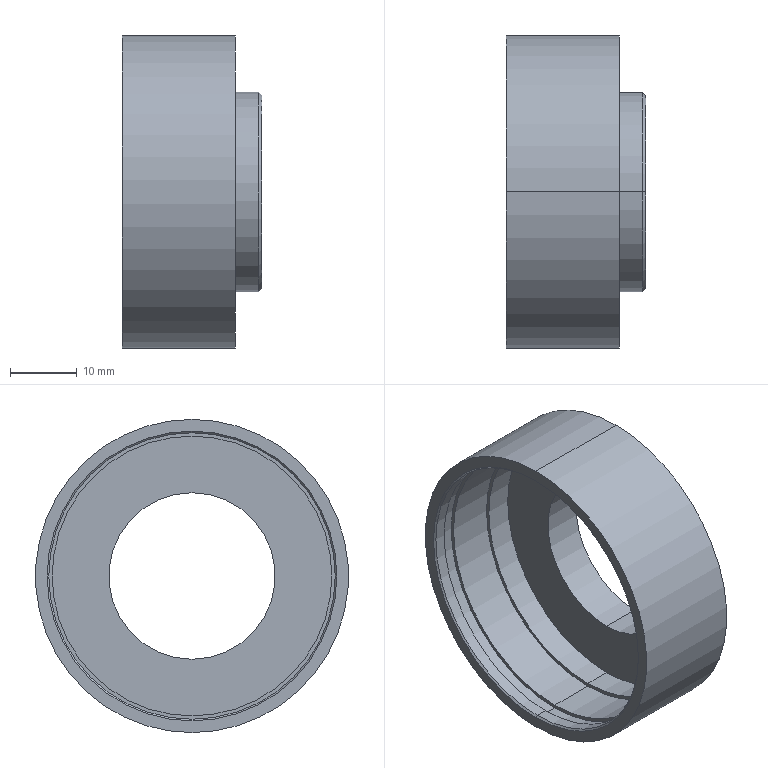Part | SolidWorks | features Chamfer 2, Revolution 1 | 1 solid | 25 faces | box 21 x 47 x 47 mm | volume 7708 mm3 | cylinder 14 | plane 7 | cone 4 | commonest cylinder face diameters 43 x4 25 x2 30 x2 42 x2 44 x2 47 x2
STEP:
#1=CARTESIAN_POINT('',(23.18,0.,-14.5));
#2=VERTEX_POINT('',#1);
#3=CARTESIAN_POINT('',(23.18,0.,14.5));
#4=VERTEX_POINT('',#3);
#5=CARTESIAN_POINT('',(23.18,0.,0.));
#6=DIRECTION('',(1.,0.,0.));
#7=DIRECTION('',(0.,0.,1.));
#8=AXIS2_PLACEMENT_3D('',#5,#6,#7);
#9=CIRCLE('',#8,14.5);
#10=EDGE_CURVE('',#2,#4,#9,.T.);
#11=ORIENTED_EDGE('',*,*,#10,.F.);
#12=CARTESIAN_POINT('',(22.68,0.,-15.));
#13=VERTEX_POINT('',#12);
#14=CARTESIAN_POINT('',(22.68,0.,-15.));
#15=DIRECTION('',(-0.7071,0.,-0.7071));
#16=VECTOR('',#15,1000.);
#17=LINE('',#14,#16);
#18=EDGE_CURVE('',#2,#13,#17,.T.);
#19=ORIENTED_EDGE('',*,*,#18,.T.);
#20=CARTESIAN_POINT('',(22.68,0.,15.));
#21=VERTEX_POINT('',#20);
#22=CARTESIAN_POINT('',(22.68,0.,0.));
#23=DIRECTION('',(-1.,0.,0.));
#24=DIRECTION('',(0.,0.,1.));
#25=AXIS2_PLACEMENT_3D('',#22,#23,#24);
#26=CIRCLE('',#25,15.);
#27=EDGE_CURVE('',#21,#13,#26,.T.);
#28=ORIENTED_EDGE('',*,*,#27,.F.);
#29=CARTESIAN_POINT('',(22.68,0.,15.));
#30=DIRECTION('',(-0.7071,0.,0.7071));
#31=VECTOR('',#30,1000.);
#32=LINE('',#29,#31);
#33=EDGE_CURVE('',#4,#21,#32,.T.);
#34=ORIENTED_EDGE('',*,*,#33,.F.);
#35=EDGE_LOOP('',(#11,#19,#28,#34));
#36=FACE_OUTER_BOUND('',#35,.T.);
#37=CARTESIAN_POINT('',(22.68,0.,0.));
#38=DIRECTION('',(-1.,0.,0.));
#39=DIRECTION('',(0.,0.,1.));
#40=AXIS2_PLACEMENT_3D('',#37,#38,#39);
#41=CONICAL_SURFACE('',#40,15.,0.7854);
#42=ADVANCED_FACE('',(#36),#41,.T.);
#43=CARTESIAN_POINT('',(2.43,0.,-21.5));
#44=VERTEX_POINT('',#43);
#45=CARTESIAN_POINT('',(2.43,0.,21.5));
#46=VERTEX_POINT('',#45);
#47=CARTESIAN_POINT('',(2.43,0.,0.));
#48=DIRECTION('',(-1.,0.,0.));
#49=DIRECTION('',(0.,0.,-1.));
#50=AXIS2_PLACEMENT_3D('',#47,#48,#49);
#51=CIRCLE('',#50,21.5);
#52=EDGE_CURVE('',#44,#46,#51,.T.);
#53=ORIENTED_EDGE('',*,*,#52,.F.);
#54=CARTESIAN_POINT('',(2.18,0.,-21.75));
#55=VERTEX_POINT('',#54);
#56=CARTESIAN_POINT('',(2.43,0.,-21.5));
#57=DIRECTION('',(-0.7071,0.,-0.7071));
#58=VECTOR('',#57,1000.);
#59=LINE('',#56,#58);
#60=EDGE_CURVE('',#44,#55,#59,.T.);
#61=ORIENTED_EDGE('',*,*,#60,.T.);
#62=CARTESIAN_POINT('',(2.18,0.,21.75));
#63=VERTEX_POINT('',#62);
#64=CARTESIAN_POINT('',(2.18,0.,0.));
#65=DIRECTION('',(1.,0.,0.));
#66=DIRECTION('',(0.,0.,-1.));
#67=AXIS2_PLACEMENT_3D('',#64,#65,#66);
#68=CIRCLE('',#67,21.75);
#69=EDGE_CURVE('',#63,#55,#68,.T.);
#70=ORIENTED_EDGE('',*,*,#69,.F.);
#71=CARTESIAN_POINT('',(2.43,0.,21.5));
#72=DIRECTION('',(-0.7071,0.,0.7071));
#73=VECTOR('',#72,1000.);
#74=LINE('',#71,#73);
#75=EDGE_CURVE('',#46,#63,#74,.T.);
#76=ORIENTED_EDGE('',*,*,#75,.F.);
#77=EDGE_LOOP('',(#53,#61,#70,#76));
#78=FACE_OUTER_BOUND('',#77,.T.);
#79=CARTESIAN_POINT('',(2.43,0.,0.));
#80=DIRECTION('',(-1.,0.,0.));
#81=DIRECTION('',(0.,0.,1.));
#82=AXIS2_PLACEMENT_3D('',#79,#80,#81);
#83=CONICAL_SURFACE('',#82,21.5,0.7854);
#84=ADVANCED_FACE('',(#78),#83,.F.);
#85=CARTESIAN_POINT('',(19.18,0.,23.5));
#86=VERTEX_POINT('',#85);
#87=CARTESIAN_POINT('',(19.18,0.,-23.5));
#88=VERTEX_POINT('',#87);
#89=CARTESIAN_POINT('',(19.18,0.,0.));
#90=DIRECTION('',(-1.,0.,0.));
#91=DIRECTION('',(0.,0.,1.));
#92=AXIS2_PLACEMENT_3D('',#89,#90,#91);
#93=CIRCLE('',#92,23.5);
#94=EDGE_CURVE('',#86,#88,#93,.T.);
#95=ORIENTED_EDGE('',*,*,#94,.T.);
#96=CARTESIAN_POINT('',(2.18,0.,-23.5));
#97=VERTEX_POINT('',#96);
#98=CARTESIAN_POINT('',(0.,0.,-23.5));
#99=DIRECTION('',(-1.,0.,0.));
#100=VECTOR('',#99,1000.);
#101=LINE('',#98,#100);
#102=EDGE_CURVE('',#88,#97,#101,.T.);
#103=ORIENTED_EDGE('',*,*,#102,.T.);
#104=CARTESIAN_POINT('',(2.18,0.,23.5));
#105=VERTEX_POINT('',#104);
#106=CARTESIAN_POINT('',(2.18,0.,0.));
#107=DIRECTION('',(-1.,0.,0.));
#108=DIRECTION('',(0.,0.,1.));
#109=AXIS2_PLACEMENT_3D('',#106,#107,#108);
#110=CIRCLE('',#109,23.5);
#111=EDGE_CURVE('',#105,#97,#110,.T.);
#112=ORIENTED_EDGE('',*,*,#111,.F.);
#113=CARTESIAN_POINT('',(0.,0.,23.5));
#114=DIRECTION('',(-1.,0.,0.));
#115=VECTOR('',#114,1000.);
#116=LINE('',#113,#115);
#117=EDGE_CURVE('',#86,#105,#116,.T.);
#118=ORIENTED_EDGE('',*,*,#117,.F.);
#119=EDGE_LOOP('',(#95,#103,#112,#118));
#120=FACE_OUTER_BOUND('',#119,.T.);
#121=CARTESIAN_POINT('',(0.,0.,0.));
#122=DIRECTION('',(-1.,0.,0.));
#123=DIRECTION('',(0.,0.,1.));
#124=AXIS2_PLACEMENT_3D('',#121,#122,#123);
#125=CYLINDRICAL_SURFACE('',#124,23.5);
#126=ADVANCED_FACE('',(#120),#125,.T.);
#127=ORIENTED_EDGE('',*,*,#27,.T.);
#128=CARTESIAN_POINT('',(19.18,0.,-15.));
#129=VERTEX_POINT('',#128);
#130=CARTESIAN_POINT('',(0.,0.,-15.));
#131=DIRECTION('',(-1.,0.,0.));
#132=VECTOR('',#131,1000.);
#133=LINE('',#130,#132);
#134=EDGE_CURVE('',#13,#129,#133,.T.);
#135=ORIENTED_EDGE('',*,*,#134,.T.);
#136=CARTESIAN_POINT('',(19.18,0.,15.));
#137=VERTEX_POINT('',#136);
#138=CARTESIAN_POINT('',(19.18,0.,0.));
#139=DIRECTION('',(-1.,0.,0.));
#140=DIRECTION('',(0.,0.,1.));
#141=AXIS2_PLACEMENT_3D('',#138,#139,#140);
#142=CIRCLE('',#141,15.);
#143=EDGE_CURVE('',#137,#129,#142,.T.);
#144=ORIENTED_EDGE('',*,*,#143,.F.);
#145=CARTESIAN_POINT('',(0.,0.,15.));
#146=DIRECTION('',(-1.,0.,0.));
#147=VECTOR('',#146,1000.);
#148=LINE('',#145,#147);
#149=EDGE_CURVE('',#21,#137,#148,.T.);
#150=ORIENTED_EDGE('',*,*,#149,.F.);
#151=EDGE_LOOP('',(#127,#135,#144,#150));
#152=FACE_OUTER_BOUND('',#151,.T.);
#153=CARTESIAN_POINT('',(0.,0.,0.));
#154=DIRECTION('',(-1.,0.,0.));
#155=DIRECTION('',(0.,0.,1.));
#156=AXIS2_PLACEMENT_3D('',#153,#154,#155);
#157=CYLINDRICAL_SURFACE('',#156,15.);
#158=ADVANCED_FACE('',(#152),#157,.T.);
#159=CARTESIAN_POINT('',(23.18,0.,-12.5));
#160=VERTEX_POINT('',#159);
#161=CARTESIAN_POINT('',(23.18,0.,12.5));
#162=VERTEX_POINT('',#161);
#163=CARTESIAN_POINT('',(23.18,0.,0.));
#164=DIRECTION('',(-1.,0.,0.));
#165=DIRECTION('',(0.,0.,1.));
#166=AXIS2_PLACEMENT_3D('',#163,#164,#165);
#167=CIRCLE('',#166,12.5);
#168=EDGE_CURVE('',#160,#162,#167,.T.);
#169=ORIENTED_EDGE('',*,*,#168,.F.);
#170=CARTESIAN_POINT('',(17.18,0.,-12.5));
#171=VERTEX_POINT('',#170);
#172=CARTESIAN_POINT('',(0.,0.,-12.5));
#173=DIRECTION('',(-1.,0.,0.));
#174=VECTOR('',#173,1000.);
#175=LINE('',#172,#174);
#176=EDGE_CURVE('',#160,#171,#175,.T.);
#177=ORIENTED_EDGE('',*,*,#176,.T.);
#178=CARTESIAN_POINT('',(17.18,0.,12.5));
#179=VERTEX_POINT('',#178);
#180=CARTESIAN_POINT('',(17.18,0.,0.));
#181=DIRECTION('',(-1.,0.,0.));
#182=DIRECTION('',(0.,0.,1.));
#183=AXIS2_PLACEMENT_3D('',#180,#181,#182);
#184=CIRCLE('',#183,12.5);
#185=EDGE_CURVE('',#171,#179,#184,.T.);
#186=ORIENTED_EDGE('',*,*,#185,.T.);
#187=CARTESIAN_POINT('',(0.,0.,12.5));
#188=DIRECTION('',(-1.,0.,0.));
#189=VECTOR('',#188,1000.);
#190=LINE('',#187,#189);
#191=EDGE_CURVE('',#162,#179,#190,.T.);
#192=ORIENTED_EDGE('',*,*,#191,.F.);
#193=EDGE_LOOP('',(#169,#177,#186,#192));
#194=FACE_OUTER_BOUND('',#193,.T.);
#195=CARTESIAN_POINT('',(0.,0.,0.));
#196=DIRECTION('',(-1.,0.,0.));
#197=DIRECTION('',(0.,0.,1.));
#198=AXIS2_PLACEMENT_3D('',#195,#196,#197);
#199=CYLINDRICAL_SURFACE('',#198,12.5);
#200=ADVANCED_FACE('',(#194),#199,.F.);
#201=CARTESIAN_POINT('',(17.18,0.,-21.));
#202=VERTEX_POINT('',#201);
#203=CARTESIAN_POINT('',(17.18,0.,21.));
#204=VERTEX_POINT('',#203);
#205=CARTESIAN_POINT('',(17.18,0.,0.));
#206=DIRECTION('',(-1.,0.,0.));
#207=DIRECTION('',(0.,0.,1.));
#208=AXIS2_PLACEMENT_3D('',#205,#206,#207);
#209=CIRCLE('',#208,21.);
#210=EDGE_CURVE('',#202,#204,#209,.T.);
#211=ORIENTED_EDGE('',*,*,#210,.F.);
#212=CARTESIAN_POINT('',(13.18,0.,-21.));
#213=VERTEX_POINT('',#212);
#214=CARTESIAN_POINT('',(0.,0.,-21.));
#215=DIRECTION('',(-1.,0.,0.));
#216=VECTOR('',#215,1000.);
#217=LINE('',#214,#216);
#218=EDGE_CURVE('',#202,#213,#217,.T.);
#219=ORIENTED_EDGE('',*,*,#218,.T.);
#220=CARTESIAN_POINT('',(13.18,0.,21.));
#221=VERTEX_POINT('',#220);
#222=CARTESIAN_POINT('',(13.18,0.,0.));
#223=DIRECTION('',(-1.,0.,0.));
#224=DIRECTION('',(0.,0.,1.));
#225=AXIS2_PLACEMENT_3D('',#222,#223,#224);
#226=CIRCLE('',#225,21.);
#227=EDGE_CURVE('',#213,#221,#226,.T.);
#228=ORIENTED_EDGE('',*,*,#227,.T.);
#229=CARTESIAN_POINT('',(0.,0.,21.));
#230=DIRECTION('',(-1.,0.,0.));
#231=VECTOR('',#230,1000.);
#232=LINE('',#229,#231);
#233=EDGE_CURVE('',#204,#221,#232,.T.);
#234=ORIENTED_EDGE('',*,*,#233,.F.);
#235=EDGE_LOOP('',(#211,#219,#228,#234));
#236=FACE_OUTER_BOUND('',#235,.T.);
#237=CARTESIAN_POINT('',(0.,0.,0.));
#238=DIRECTION('',(-1.,0.,0.));
#239=DIRECTION('',(0.,0.,1.));
#240=AXIS2_PLACEMENT_3D('',#237,#238,#239);
#241=CYLINDRICAL_SURFACE('',#240,21.);
#242=ADVANCED_FACE('',(#236),#241,.F.);
#243=CARTESIAN_POINT('',(13.18,0.,-21.5));
#244=VERTEX_POINT('',#243);
#245=CARTESIAN_POINT('',(13.18,0.,21.5));
#246=VERTEX_POINT('',#245);
#247=CARTESIAN_POINT('',(13.18,0.,0.));
#248=DIRECTION('',(-1.,0.,0.));
#249=DIRECTION('',(0.,0.,1.));
#250=AXIS2_PLACEMENT_3D('',#247,#248,#249);
#251=CIRCLE('',#250,21.5);
#252=EDGE_CURVE('',#244,#246,#251,.T.);
#253=ORIENTED_EDGE('',*,*,#252,.F.);
#254=CARTESIAN_POINT('',(6.18,0.,-21.5));
#255=VERTEX_POINT('',#254);
#256=CARTESIAN_POINT('',(0.,0.,-21.5));
#257=DIRECTION('',(-1.,0.,0.));
#258=VECTOR('',#257,1000.);
#259=LINE('',#256,#258);
#260=EDGE_CURVE('',#244,#255,#259,.T.);
#261=ORIENTED_EDGE('',*,*,#260,.T.);
#262=CARTESIAN_POINT('',(6.18,0.,21.5));
#263=VERTEX_POINT('',#262);
#264=CARTESIAN_POINT('',(6.18,0.,0.));
#265=DIRECTION('',(-1.,0.,0.));
#266=DIRECTION('',(0.,0.,1.));
#267=AXIS2_PLACEMENT_3D('',#264,#265,#266);
#268=CIRCLE('',#267,21.5);
#269=EDGE_CURVE('',#255,#263,#268,.T.);
#270=ORIENTED_EDGE('',*,*,#269,.T.);
#271=CARTESIAN_POINT('',(0.,0.,21.5));
#272=DIRECTION('',(-1.,0.,0.));
#273=VECTOR('',#272,1000.);
#274=LINE('',#271,#273);
#275=EDGE_CURVE('',#246,#263,#274,.T.);
#276=ORIENTED_EDGE('',*,*,#275,.F.);
#277=EDGE_LOOP('',(#253,#261,#270,#276));
#278=FACE_OUTER_BOUND('',#277,.T.);
#279=CARTESIAN_POINT('',(0.,0.,0.));
#280=DIRECTION('',(-1.,0.,0.));
#281=DIRECTION('',(0.,0.,1.));
#282=AXIS2_PLACEMENT_3D('',#279,#280,#281);
#283=CYLINDRICAL_SURFACE('',#282,21.5);
#284=ADVANCED_FACE('',(#278),#283,.F.);
#285=CARTESIAN_POINT('',(6.18,0.,-22.));
#286=VERTEX_POINT('',#285);
#287=CARTESIAN_POINT('',(6.18,0.,22.));
#288=VERTEX_POINT('',#287);
#289=CARTESIAN_POINT('',(6.18,0.,0.));
#290=DIRECTION('',(-1.,0.,0.));
#291=DIRECTION('',(0.,0.,1.));
#292=AXIS2_PLACEMENT_3D('',#289,#290,#291);
#293=CIRCLE('',#292,22.);
#294=EDGE_CURVE('',#286,#288,#293,.T.);
#295=ORIENTED_EDGE('',*,*,#294,.F.);
#296=CARTESIAN_POINT('',(4.18,0.,-22.));
#297=VERTEX_POINT('',#296);
#298=CARTESIAN_POINT('',(0.,0.,-22.));
#299=DIRECTION('',(-1.,0.,0.));
#300=VECTOR('',#299,1000.);
#301=LINE('',#298,#300);
#302=EDGE_CURVE('',#286,#297,#301,.T.);
#303=ORIENTED_EDGE('',*,*,#302,.T.);
#304=CARTESIAN_POINT('',(4.18,0.,22.));
#305=VERTEX_POINT('',#304);
#306=CARTESIAN_POINT('',(4.18,0.,0.));
#307=DIRECTION('',(-1.,0.,0.));
#308=DIRECTION('',(0.,0.,1.));
#309=AXIS2_PLACEMENT_3D('',#306,#307,#308);
#310=CIRCLE('',#309,22.);
#311=EDGE_CURVE('',#297,#305,#310,.T.);
#312=ORIENTED_EDGE('',*,*,#311,.T.);
#313=CARTESIAN_POINT('',(0.,0.,22.));
#314=DIRECTION('',(-1.,0.,0.));
#315=VECTOR('',#314,1000.);
#316=LINE('',#313,#315);
#317=EDGE_CURVE('',#288,#305,#316,.T.);
#318=ORIENTED_EDGE('',*,*,#317,.F.);
#319=EDGE_LOOP('',(#295,#303,#312,#318));
#320=FACE_OUTER_BOUND('',#319,.T.);
#321=CARTESIAN_POINT('',(0.,0.,0.));
#322=DIRECTION('',(-1.,0.,0.));
#323=DIRECTION('',(0.,0.,1.));
#324=AXIS2_PLACEMENT_3D('',#321,#322,#323);
#325=CYLINDRICAL_SURFACE('',#324,22.);
#326=ADVANCED_FACE('',(#320),#325,.F.);
#327=CARTESIAN_POINT('',(4.18,0.,-21.5));
#328=VERTEX_POINT('',#327);
#329=CARTESIAN_POINT('',(4.18,0.,21.5));
#330=VERTEX_POINT('',#329);
#331=CARTESIAN_POINT('',(4.18,0.,0.));
#332=DIRECTION('',(-1.,0.,0.));
#333=DIRECTION('',(0.,0.,1.));
#334=AXIS2_PLACEMENT_3D('',#331,#332,#333);
#335=CIRCLE('',#334,21.5);
#336=EDGE_CURVE('',#328,#330,#335,.T.);
#337=ORIENTED_EDGE('',*,*,#336,.F.);
#338=CARTESIAN_POINT('',(0.,0.,-21.5));
#339=DIRECTION('',(-1.,0.,0.));
#340=VECTOR('',#339,1000.);
#341=LINE('',#338,#340);
#342=EDGE_CURVE('',#328,#44,#341,.T.);
#343=ORIENTED_EDGE('',*,*,#342,.T.);
#344=ORIENTED_EDGE('',*,*,#52,.T.);
#345=CARTESIAN_POINT('',(0.,0.,21.5));
#346=DIRECTION('',(-1.,0.,0.));
#347=VECTOR('',#346,1000.);
#348=LINE('',#345,#347);
#349=EDGE_CURVE('',#330,#46,#348,.T.);
#350=ORIENTED_EDGE('',*,*,#349,.F.);
#351=EDGE_LOOP('',(#337,#343,#344,#350));
#352=FACE_OUTER_BOUND('',#351,.T.);
#353=CARTESIAN_POINT('',(0.,0.,0.));
#354=DIRECTION('',(-1.,0.,0.));
#355=DIRECTION('',(0.,0.,1.));
#356=AXIS2_PLACEMENT_3D('',#353,#354,#355);
#357=CYLINDRICAL_SURFACE('',#356,21.5);
#358=ADVANCED_FACE('',(#352),#357,.F.);
#359=ORIENTED_EDGE('',*,*,#69,.T.);
#360=CARTESIAN_POINT('',(2.18,0.,0.));
#361=DIRECTION('',(1.,0.,0.));
#362=DIRECTION('',(0.,0.,-1.));
#363=AXIS2_PLACEMENT_3D('',#360,#361,#362);
#364=CIRCLE('',#363,21.75);
#365=EDGE_CURVE('',#55,#63,#364,.T.);
#366=ORIENTED_EDGE('',*,*,#365,.T.);
#367=EDGE_LOOP('',(#359,#366));
#368=FACE_BOUND('',#367,.T.);
#369=ORIENTED_EDGE('',*,*,#111,.T.);
#370=CARTESIAN_POINT('',(2.18,0.,0.));
#371=DIRECTION('',(-1.,0.,0.));
#372=DIRECTION('',(0.,0.,1.));
#373=AXIS2_PLACEMENT_3D('',#370,#371,#372);
#374=CIRCLE('',#373,23.5);
#375=EDGE_CURVE('',#97,#105,#374,.T.);
#376=ORIENTED_EDGE('',*,*,#375,.T.);
#377=EDGE_LOOP('',(#369,#376));
#378=FACE_OUTER_BOUND('',#377,.T.);
#379=CARTESIAN_POINT('',(2.18,23.5,0.));
#380=DIRECTION('',(1.,0.,0.));
#381=DIRECTION('',(0.,0.,-1.));
#382=AXIS2_PLACEMENT_3D('',#379,#380,#381);
#383=PLANE('',#382);
#384=ADVANCED_FACE('',(#368,#378),#383,.F.);
#385=ORIENTED_EDGE('',*,*,#342,.F.);
#386=CARTESIAN_POINT('',(4.18,0.,0.));
#387=DIRECTION('',(-1.,0.,0.));
#388=DIRECTION('',(0.,0.,1.));
#389=AXIS2_PLACEMENT_3D('',#386,#387,#388);
#390=CIRCLE('',#389,21.5);
#391=EDGE_CURVE('',#330,#328,#390,.T.);
#392=ORIENTED_EDGE('',*,*,#391,.F.);
#393=ORIENTED_EDGE('',*,*,#349,.T.);
#394=CARTESIAN_POINT('',(2.43,0.,0.));
#395=DIRECTION('',(-1.,0.,0.));
#396=DIRECTION('',(0.,0.,-1.));
#397=AXIS2_PLACEMENT_3D('',#394,#395,#396);
#398=CIRCLE('',#397,21.5);
#399=EDGE_CURVE('',#46,#44,#398,.T.);
#400=ORIENTED_EDGE('',*,*,#399,.T.);
#401=EDGE_LOOP('',(#385,#392,#393,#400));
#402=FACE_OUTER_BOUND('',#401,.T.);
#403=CARTESIAN_POINT('',(0.,0.,0.));
#404=DIRECTION('',(-1.,0.,0.));
#405=DIRECTION('',(0.,0.,1.));
#406=AXIS2_PLACEMENT_3D('',#403,#404,#405);
#407=CYLINDRICAL_SURFACE('',#406,21.5);
#408=ADVANCED_FACE('',(#402),#407,.F.);
#409=CARTESIAN_POINT('',(4.18,0.,0.));
#410=DIRECTION('',(-1.,0.,0.));
#411=DIRECTION('',(0.,0.,1.));
#412=AXIS2_PLACEMENT_3D('',#409,#410,#411);
#413=CIRCLE('',#412,22.);
#414=EDGE_CURVE('',#305,#297,#413,.T.);
#415=ORIENTED_EDGE('',*,*,#414,.F.);
#416=ORIENTED_EDGE('',*,*,#311,.F.);
#417=EDGE_LOOP('',(#415,#416));
#418=FACE_OUTER_BOUND('',#417,.T.);
#419=ORIENTED_EDGE('',*,*,#391,.T.);
#420=ORIENTED_EDGE('',*,*,#336,.T.);
#421=EDGE_LOOP('',(#419,#420));
#422=FACE_BOUND('',#421,.T.);
#423=CARTESIAN_POINT('',(4.18,22.,0.));
#424=DIRECTION('',(-1.,0.,0.));
#425=DIRECTION('',(0.,0.,1.));
#426=AXIS2_PLACEMENT_3D('',#423,#424,#425);
#427=PLANE('',#426);
#428=ADVANCED_FACE('',(#418,#422),#427,.F.);
#429=ORIENTED_EDGE('',*,*,#302,.F.);
#430=CARTESIAN_POINT('',(6.18,0.,0.));
#431=DIRECTION('',(-1.,0.,0.));
#432=DIRECTION('',(0.,0.,1.));
#433=AXIS2_PLACEMENT_3D('',#430,#431,#432);
#434=CIRCLE('',#433,22.);
#435=EDGE_CURVE('',#288,#286,#434,.T.);
#436=ORIENTED_EDGE('',*,*,#435,.F.);
#437=ORIENTED_EDGE('',*,*,#317,.T.);
#438=ORIENTED_EDGE('',*,*,#414,.T.);
#439=EDGE_LOOP('',(#429,#436,#437,#438));
#440=FACE_OUTER_BOUND('',#439,.T.);
#441=CARTESIAN_POINT('',(0.,0.,0.));
#442=DIRECTION('',(-1.,0.,0.));
#443=DIRECTION('',(0.,0.,1.));
#444=AXIS2_PLACEMENT_3D('',#441,#442,#443);
#445=CYLINDRICAL_SURFACE('',#444,22.);
#446=ADVANCED_FACE('',(#440),#445,.F.);
#447=CARTESIAN_POINT('',(6.18,0.,0.));
#448=DIRECTION('',(-1.,0.,0.));
#449=DIRECTION('',(0.,0.,1.));
#450=AXIS2_PLACEMENT_3D('',#447,#448,#449);
#451=CIRCLE('',#450,21.5);
#452=EDGE_CURVE('',#263,#255,#451,.T.);
#453=ORIENTED_EDGE('',*,*,#452,.F.);
#454=ORIENTED_EDGE('',*,*,#269,.F.);
#455=EDGE_LOOP('',(#453,#454));
#456=FACE_BOUND('',#455,.T.);
#457=ORIENTED_EDGE('',*,*,#435,.T.);
#458=ORIENTED_EDGE('',*,*,#294,.T.);
#459=EDGE_LOOP('',(#457,#458));
#460=FACE_OUTER_BOUND('',#459,.T.);
#461=CARTESIAN_POINT('',(6.18,22.,0.));
#462=DIRECTION('',(1.,0.,0.));
#463=DIRECTION('',(0.,0.,-1.));
#464=AXIS2_PLACEMENT_3D('',#461,#462,#463);
#465=PLANE('',#464);
#466=ADVANCED_FACE('',(#456,#460),#465,.F.);
#467=ORIENTED_EDGE('',*,*,#260,.F.);
#468=CARTESIAN_POINT('',(13.18,0.,0.));
#469=DIRECTION('',(-1.,0.,0.));
#470=DIRECTION('',(0.,0.,1.));
#471=AXIS2_PLACEMENT_3D('',#468,#469,#470);
#472=CIRCLE('',#471,21.5);
#473=EDGE_CURVE('',#246,#244,#472,.T.);
#474=ORIENTED_EDGE('',*,*,#473,.F.);
#475=ORIENTED_EDGE('',*,*,#275,.T.);
#476=ORIENTED_EDGE('',*,*,#452,.T.);
#477=EDGE_LOOP('',(#467,#474,#475,#476));
#478=FACE_OUTER_BOUND('',#477,.T.);
#479=CARTESIAN_POINT('',(0.,0.,0.));
#480=DIRECTION('',(-1.,0.,0.));
#481=DIRECTION('',(0.,0.,1.));
#482=AXIS2_PLACEMENT_3D('',#479,#480,#481);
#483=CYLINDRICAL_SURFACE('',#482,21.5);
#484=ADVANCED_FACE('',(#478),#483,.F.);
#485=CARTESIAN_POINT('',(13.18,0.,0.));
#486=DIRECTION('',(-1.,0.,0.));
#487=DIRECTION('',(0.,0.,1.));
#488=AXIS2_PLACEMENT_3D('',#485,#486,#487);
#489=CIRCLE('',#488,21.);
#490=EDGE_CURVE('',#221,#213,#489,.T.);
#491=ORIENTED_EDGE('',*,*,#490,.F.);
#492=ORIENTED_EDGE('',*,*,#227,.F.);
#493=EDGE_LOOP('',(#491,#492));
#494=FACE_BOUND('',#493,.T.);
#495=ORIENTED_EDGE('',*,*,#473,.T.);
#496=ORIENTED_EDGE('',*,*,#252,.T.);
#497=EDGE_LOOP('',(#495,#496));
#498=FACE_OUTER_BOUND('',#497,.T.);
#499=CARTESIAN_POINT('',(13.18,21.5,0.));
#500=DIRECTION('',(1.,0.,0.));
#501=DIRECTION('',(0.,0.,-1.));
#502=AXIS2_PLACEMENT_3D('',#499,#500,#501);
#503=PLANE('',#502);
#504=ADVANCED_FACE('',(#494,#498),#503,.F.);
#505=ORIENTED_EDGE('',*,*,#218,.F.);
#506=CARTESIAN_POINT('',(17.18,0.,0.));
#507=DIRECTION('',(-1.,0.,0.));
#508=DIRECTION('',(0.,0.,1.));
#509=AXIS2_PLACEMENT_3D('',#506,#507,#508);
#510=CIRCLE('',#509,21.);
#511=EDGE_CURVE('',#204,#202,#510,.T.);
#512=ORIENTED_EDGE('',*,*,#511,.F.);
#513=ORIENTED_EDGE('',*,*,#233,.T.);
#514=ORIENTED_EDGE('',*,*,#490,.T.);
#515=EDGE_LOOP('',(#505,#512,#513,#514));
#516=FACE_OUTER_BOUND('',#515,.T.);
#517=CARTESIAN_POINT('',(0.,0.,0.));
#518=DIRECTION('',(-1.,0.,0.));
#519=DIRECTION('',(0.,0.,1.));
#520=AXIS2_PLACEMENT_3D('',#517,#518,#519);
#521=CYLINDRICAL_SURFACE('',#520,21.);
#522=ADVANCED_FACE('',(#516),#521,.F.);
#523=CARTESIAN_POINT('',(17.18,0.,0.));
#524=DIRECTION('',(-1.,0.,0.));
#525=DIRECTION('',(0.,0.,1.));
#526=AXIS2_PLACEMENT_3D('',#523,#524,#525);
#527=CIRCLE('',#526,12.5);
#528=EDGE_CURVE('',#179,#171,#527,.T.);
#529=ORIENTED_EDGE('',*,*,#528,.F.);
#530=ORIENTED_EDGE('',*,*,#185,.F.);
#531=EDGE_LOOP('',(#529,#530));
#532=FACE_BOUND('',#531,.T.);
#533=ORIENTED_EDGE('',*,*,#511,.T.);
#534=ORIENTED_EDGE('',*,*,#210,.T.);
#535=EDGE_LOOP('',(#533,#534));
#536=FACE_OUTER_BOUND('',#535,.T.);
#537=CARTESIAN_POINT('',(17.18,21.,0.));
#538=DIRECTION('',(1.,0.,0.));
#539=DIRECTION('',(0.,0.,-1.));
#540=AXIS2_PLACEMENT_3D('',#537,#538,#539);
#541=PLANE('',#540);
#542=ADVANCED_FACE('',(#532,#536),#541,.F.);
#543=ORIENTED_EDGE('',*,*,#176,.F.);
#544=CARTESIAN_POINT('',(23.18,0.,0.));
#545=DIRECTION('',(-1.,0.,0.));
#546=DIRECTION('',(0.,0.,1.));
#547=AXIS2_PLACEMENT_3D('',#544,#545,#546);
#548=CIRCLE('',#547,12.5);
#549=EDGE_CURVE('',#162,#160,#548,.T.);
#550=ORIENTED_EDGE('',*,*,#549,.F.);
#551=ORIENTED_EDGE('',*,*,#191,.T.);
#552=ORIENTED_EDGE('',*,*,#528,.T.);
#553=EDGE_LOOP('',(#543,#550,#551,#552));
#554=FACE_OUTER_BOUND('',#553,.T.);
#555=CARTESIAN_POINT('',(0.,0.,0.));
#556=DIRECTION('',(-1.,0.,0.));
#557=DIRECTION('',(0.,0.,1.));
#558=AXIS2_PLACEMENT_3D('',#555,#556,#557);
#559=CYLINDRICAL_SURFACE('',#558,12.5);
#560=ADVANCED_FACE('',(#554),#559,.F.);
#561=CARTESIAN_POINT('',(23.18,0.,0.));
#562=DIRECTION('',(1.,0.,0.));
#563=DIRECTION('',(0.,0.,1.));
#564=AXIS2_PLACEMENT_3D('',#561,#562,#563);
#565=CIRCLE('',#564,14.5);
#566=EDGE_CURVE('',#4,#2,#565,.T.);
#567=ORIENTED_EDGE('',*,*,#566,.T.);
#568=ORIENTED_EDGE('',*,*,#10,.T.);
#569=EDGE_LOOP('',(#567,#568));
#570=FACE_OUTER_BOUND('',#569,.T.);
#571=ORIENTED_EDGE('',*,*,#549,.T.);
#572=ORIENTED_EDGE('',*,*,#168,.T.);
#573=EDGE_LOOP('',(#571,#572));
#574=FACE_BOUND('',#573,.T.);
#575=CARTESIAN_POINT('',(23.18,12.5,0.));
#576=DIRECTION('',(-1.,0.,0.));
#577=DIRECTION('',(0.,0.,1.));
#578=AXIS2_PLACEMENT_3D('',#575,#576,#577);
#579=PLANE('',#578);
#580=ADVANCED_FACE('',(#570,#574),#579,.F.);
#581=ORIENTED_EDGE('',*,*,#134,.F.);
#582=CARTESIAN_POINT('',(22.68,0.,0.));
#583=DIRECTION('',(-1.,0.,0.));
#584=DIRECTION('',(0.,0.,1.));
#585=AXIS2_PLACEMENT_3D('',#582,#583,#584);
#586=CIRCLE('',#585,15.);
#587=EDGE_CURVE('',#13,#21,#586,.T.);
#588=ORIENTED_EDGE('',*,*,#587,.T.);
#589=ORIENTED_EDGE('',*,*,#149,.T.);
#590=CARTESIAN_POINT('',(19.18,0.,0.));
#591=DIRECTION('',(-1.,0.,0.));
#592=DIRECTION('',(0.,0.,1.));
#593=AXIS2_PLACEMENT_3D('',#590,#591,#592);
#594=CIRCLE('',#593,15.);
#595=EDGE_CURVE('',#129,#137,#594,.T.);
#596=ORIENTED_EDGE('',*,*,#595,.F.);
#597=EDGE_LOOP('',(#581,#588,#589,#596));
#598=FACE_OUTER_BOUND('',#597,.T.);
#599=CARTESIAN_POINT('',(0.,0.,0.));
#600=DIRECTION('',(-1.,0.,0.));
#601=DIRECTION('',(0.,0.,1.));
#602=AXIS2_PLACEMENT_3D('',#599,#600,#601);
#603=CYLINDRICAL_SURFACE('',#602,15.);
#604=ADVANCED_FACE('',(#598),#603,.T.);
#605=ORIENTED_EDGE('',*,*,#94,.F.);
#606=CARTESIAN_POINT('',(19.18,0.,0.));
#607=DIRECTION('',(-1.,0.,0.));
#608=DIRECTION('',(0.,0.,1.));
#609=AXIS2_PLACEMENT_3D('',#606,#607,#608);
#610=CIRCLE('',#609,23.5);
#611=EDGE_CURVE('',#88,#86,#610,.T.);
#612=ORIENTED_EDGE('',*,*,#611,.F.);
#613=EDGE_LOOP('',(#605,#612));
#614=FACE_OUTER_BOUND('',#613,.T.);
#615=ORIENTED_EDGE('',*,*,#143,.T.);
#616=ORIENTED_EDGE('',*,*,#595,.T.);
#617=EDGE_LOOP('',(#615,#616));
#618=FACE_BOUND('',#617,.T.);
#619=CARTESIAN_POINT('',(19.18,15.,0.));
#620=DIRECTION('',(-1.,0.,0.));
#621=DIRECTION('',(0.,0.,1.));
#622=AXIS2_PLACEMENT_3D('',#619,#620,#621);
#623=PLANE('',#622);
#624=ADVANCED_FACE('',(#614,#618),#623,.F.);
#625=ORIENTED_EDGE('',*,*,#102,.F.);
#626=ORIENTED_EDGE('',*,*,#611,.T.);
#627=ORIENTED_EDGE('',*,*,#117,.T.);
#628=ORIENTED_EDGE('',*,*,#375,.F.);
#629=EDGE_LOOP('',(#625,#626,#627,#628));
#630=FACE_OUTER_BOUND('',#629,.T.);
#631=CARTESIAN_POINT('',(0.,0.,0.));
#632=DIRECTION('',(-1.,0.,0.));
#633=DIRECTION('',(0.,0.,1.));
#634=AXIS2_PLACEMENT_3D('',#631,#632,#633);
#635=CYLINDRICAL_SURFACE('',#634,23.5);
#636=ADVANCED_FACE('',(#630),#635,.T.);
#637=ORIENTED_EDGE('',*,*,#60,.F.);
#638=ORIENTED_EDGE('',*,*,#399,.F.);
#639=ORIENTED_EDGE('',*,*,#75,.T.);
#640=ORIENTED_EDGE('',*,*,#365,.F.);
#641=EDGE_LOOP('',(#637,#638,#639,#640));
#642=FACE_OUTER_BOUND('',#641,.T.);
#643=CARTESIAN_POINT('',(2.43,0.,0.));
#644=DIRECTION('',(-1.,0.,0.));
#645=DIRECTION('',(0.,0.,1.));
#646=AXIS2_PLACEMENT_3D('',#643,#644,#645);
#647=CONICAL_SURFACE('',#646,21.5,0.7854);
#648=ADVANCED_FACE('',(#642),#647,.F.);
#649=ORIENTED_EDGE('',*,*,#18,.F.);
#650=ORIENTED_EDGE('',*,*,#566,.F.);
#651=ORIENTED_EDGE('',*,*,#33,.T.);
#652=ORIENTED_EDGE('',*,*,#587,.F.);
#653=EDGE_LOOP('',(#649,#650,#651,#652));
#654=FACE_OUTER_BOUND('',#653,.T.);
#655=CARTESIAN_POINT('',(22.68,0.,0.));
#656=DIRECTION('',(-1.,0.,0.));
#657=DIRECTION('',(0.,0.,1.));
#658=AXIS2_PLACEMENT_3D('',#655,#656,#657);
#659=CONICAL_SURFACE('',#658,15.,0.7854);
#660=ADVANCED_FACE('',(#654),#659,.T.);
#661=CLOSED_SHELL('',(#42,#84,#126,#158,#200,#242,#284,#326,#358,#384,#408,#428,#446,#466,#484,#504,#522,#542,#560,#580,#604,#624,#636,#648,#660));
#662=MANIFOLD_SOLID_BREP('',#661);
#663=CARTESIAN_POINT('',(0.,0.,0.));
#664=DIRECTION('',(0.,0.,1.));
#665=DIRECTION('',(1.,0.,0.));
#666=AXIS2_PLACEMENT_3D('',#663,#664,#665);
#667=(LENGTH_UNIT()NAMED_UNIT(*)SI_UNIT(.MILLI.,.METRE.));
#668=UNCERTAINTY_MEASURE_WITH_UNIT(LENGTH_MEASURE(0.00001),#667,'','');
#669=(NAMED_UNIT(*)PLANE_ANGLE_UNIT()SI_UNIT($,.RADIAN.));
#670=(NAMED_UNIT(*)SI_UNIT($,.STERADIAN.)SOLID_ANGLE_UNIT());
#671=(GEOMETRIC_REPRESENTATION_CONTEXT(3)GLOBAL_UNCERTAINTY_ASSIGNED_CONTEXT((#668))GLOBAL_UNIT_ASSIGNED_CONTEXT((#667,#669,#670))REPRESENTATION_CONTEXT('',''));
#672=ADVANCED_BREP_SHAPE_REPRESENTATION('',(#662,#666),#671);